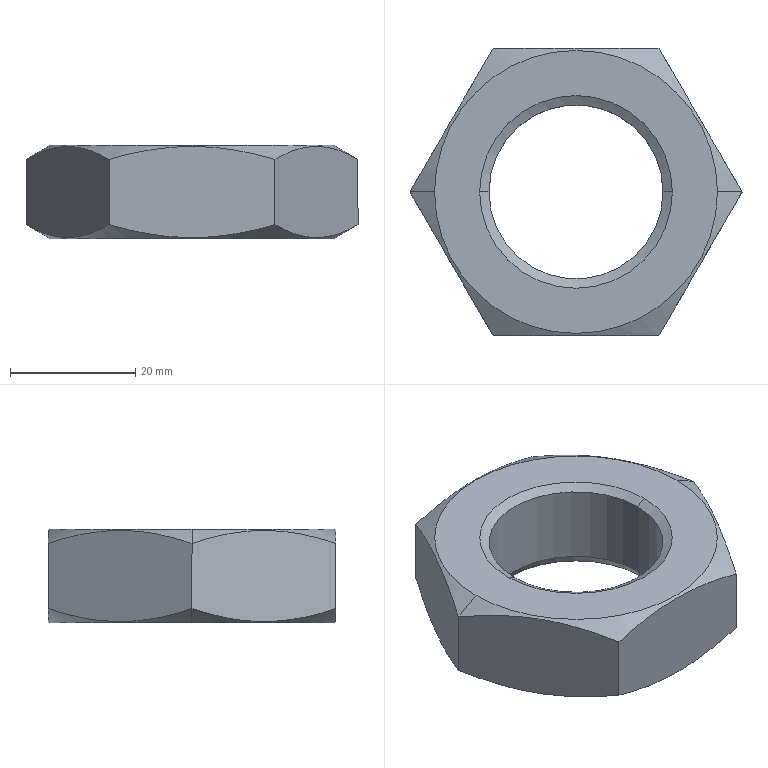Part | SolidWorks | features RevCut 2, Chamfer 1, Extrusion 1, LPattern 1 | 1 solid | 18 faces | box 53.116 x 46 x 15 mm | volume 17946 mm3 | cone 8 | plane 8 | cylinder 2 | commonest cylinder face diameters 27.835 x2
STEP:
#1=CARTESIAN_POINT('',(-13.918,0.,-0.866));
#2=VERTEX_POINT('',#1);
#3=CARTESIAN_POINT('',(13.918,0.,-0.866));
#4=VERTEX_POINT('',#3);
#5=CARTESIAN_POINT('',(0.,0.,-0.866));
#6=DIRECTION('',(0.,0.,1.));
#7=DIRECTION('',(1.,0.,0.));
#8=AXIS2_PLACEMENT_3D('',#5,#6,#7);
#9=CIRCLE('',#8,13.918);
#10=EDGE_CURVE('',#2,#4,#9,.T.);
#11=ORIENTED_EDGE('',*,*,#10,.F.);
#12=CARTESIAN_POINT('',(-15.418,0.,0.));
#13=VERTEX_POINT('',#12);
#14=CARTESIAN_POINT('',(-13.918,0.,-0.866));
#15=DIRECTION('',(-0.866,0.,0.5));
#16=VECTOR('',#15,1000.);
#17=LINE('',#14,#16);
#18=EDGE_CURVE('',#2,#13,#17,.T.);
#19=ORIENTED_EDGE('',*,*,#18,.T.);
#20=CARTESIAN_POINT('',(15.418,0.,0.));
#21=VERTEX_POINT('',#20);
#22=CARTESIAN_POINT('',(0.,0.,0.));
#23=DIRECTION('',(0.,0.,-1.));
#24=DIRECTION('',(1.,0.,0.));
#25=AXIS2_PLACEMENT_3D('',#22,#23,#24);
#26=CIRCLE('',#25,15.418);
#27=EDGE_CURVE('',#21,#13,#26,.T.);
#28=ORIENTED_EDGE('',*,*,#27,.F.);
#29=CARTESIAN_POINT('',(13.918,0.,-0.866));
#30=DIRECTION('',(0.866,0.,0.5));
#31=VECTOR('',#30,1000.);
#32=LINE('',#29,#31);
#33=EDGE_CURVE('',#4,#21,#32,.T.);
#34=ORIENTED_EDGE('',*,*,#33,.F.);
#35=EDGE_LOOP('',(#11,#19,#28,#34));
#36=FACE_OUTER_BOUND('',#35,.T.);
#37=CARTESIAN_POINT('',(0.,0.,-0.866));
#38=DIRECTION('',(0.,0.,1.));
#39=DIRECTION('',(1.,0.,0.));
#40=AXIS2_PLACEMENT_3D('',#37,#38,#39);
#41=CONICAL_SURFACE('',#40,13.918,1.047);
#42=ADVANCED_FACE('',(#36),#41,.F.);
#43=CARTESIAN_POINT('',(13.918,0.,-13.5));
#44=VERTEX_POINT('',#43);
#45=CARTESIAN_POINT('',(-13.918,0.,-13.5));
#46=VERTEX_POINT('',#45);
#47=CARTESIAN_POINT('',(0.,0.,-13.5));
#48=DIRECTION('',(0.,0.,-1.));
#49=DIRECTION('',(1.,0.,0.));
#50=AXIS2_PLACEMENT_3D('',#47,#48,#49);
#51=CIRCLE('',#50,13.918);
#52=EDGE_CURVE('',#44,#46,#51,.T.);
#53=ORIENTED_EDGE('',*,*,#52,.F.);
#54=CARTESIAN_POINT('',(14.784,0.,-15.));
#55=VERTEX_POINT('',#54);
#56=CARTESIAN_POINT('',(14.784,0.,-15.));
#57=DIRECTION('',(0.5,0.,-0.866));
#58=VECTOR('',#57,1000.);
#59=LINE('',#56,#58);
#60=EDGE_CURVE('',#44,#55,#59,.T.);
#61=ORIENTED_EDGE('',*,*,#60,.T.);
#62=CARTESIAN_POINT('',(-14.784,0.,-15.));
#63=VERTEX_POINT('',#62);
#64=CARTESIAN_POINT('',(0.,0.,-15.));
#65=DIRECTION('',(0.,0.,1.));
#66=DIRECTION('',(1.,0.,0.));
#67=AXIS2_PLACEMENT_3D('',#64,#65,#66);
#68=CIRCLE('',#67,14.784);
#69=EDGE_CURVE('',#63,#55,#68,.T.);
#70=ORIENTED_EDGE('',*,*,#69,.F.);
#71=CARTESIAN_POINT('',(-14.784,0.,-15.));
#72=DIRECTION('',(-0.5,0.,-0.866));
#73=VECTOR('',#72,1000.);
#74=LINE('',#71,#73);
#75=EDGE_CURVE('',#46,#63,#74,.T.);
#76=ORIENTED_EDGE('',*,*,#75,.F.);
#77=EDGE_LOOP('',(#53,#61,#70,#76));
#78=FACE_OUTER_BOUND('',#77,.T.);
#79=CARTESIAN_POINT('',(0.,0.,-15.));
#80=DIRECTION('',(0.,0.,-1.));
#81=DIRECTION('',(-1.,0.,0.));
#82=AXIS2_PLACEMENT_3D('',#79,#80,#81);
#83=CONICAL_SURFACE('',#82,14.784,0.5236);
#84=ADVANCED_FACE('',(#78),#83,.F.);
#85=CARTESIAN_POINT('',(-22.625,0.,0.));
#86=VERTEX_POINT('',#85);
#87=CARTESIAN_POINT('',(22.625,0.,0.));
#88=VERTEX_POINT('',#87);
#89=CARTESIAN_POINT('',(0.,0.,0.));
#90=DIRECTION('',(0.,0.,-1.));
#91=DIRECTION('',(-1.,0.,0.));
#92=AXIS2_PLACEMENT_3D('',#89,#90,#91);
#93=CIRCLE('',#92,22.625);
#94=EDGE_CURVE('',#86,#88,#93,.T.);
#95=ORIENTED_EDGE('',*,*,#94,.T.);
#96=CARTESIAN_POINT('',(26.558,0.,-2.271));
#97=VERTEX_POINT('',#96);
#98=CARTESIAN_POINT('',(22.625,0.,0.));
#99=DIRECTION('',(0.866,0.,-0.5));
#100=VECTOR('',#99,1000.);
#101=LINE('',#98,#100);
#102=EDGE_CURVE('',#88,#97,#101,.T.);
#103=ORIENTED_EDGE('',*,*,#102,.T.);
#104=CARTESIAN_POINT('',(13.279,23.,-2.271));
#105=VERTEX_POINT('',#104);
#106=CARTESIAN_POINT('',(26.558,0.,-2.271));
#107=CARTESIAN_POINT('',(25.474,1.878,-1.645));
#108=CARTESIAN_POINT('',(24.382,3.769,-1.129));
#109=CARTESIAN_POINT('',(22.175,7.591,-0.4144));
#110=CARTESIAN_POINT('',(21.06,9.523,-0.218));
#111=CARTESIAN_POINT('',(19.649,11.967,-0.2162));
#112=CARTESIAN_POINT('',(19.365,12.458,-0.2279));
#113=CARTESIAN_POINT('',(18.801,13.436,-0.2751));
#114=CARTESIAN_POINT('',(18.519,13.924,-0.3106));
#115=CARTESIAN_POINT('',(17.678,15.381,-0.4511));
#116=CARTESIAN_POINT('',(17.121,16.346,-0.5901));
#117=CARTESIAN_POINT('',(15.459,19.224,-1.127));
#118=CARTESIAN_POINT('',(14.365,21.12,-1.644));
#119=CARTESIAN_POINT('',(13.279,23.,-2.271));
#120=B_SPLINE_CURVE_WITH_KNOTS('',3,(#106,#107,#108,#109,#110,#111,#112,#113,#114,#115,#116,#117,#118,#119),.UNSPECIFIED.,.F.,.F.,(4,2,2,2,2,2,4),(0.000000238,0.006706,0.01341,0.01509,0.01676,0.02012,0.02682),.UNSPECIFIED.);
#121=EDGE_CURVE('',#97,#105,#120,.T.);
#122=ORIENTED_EDGE('',*,*,#121,.T.);
#123=CARTESIAN_POINT('',(-13.279,23.,-2.271));
#124=VERTEX_POINT('',#123);
#125=CARTESIAN_POINT('',(13.279,23.,-2.271));
#126=CARTESIAN_POINT('',(11.133,23.,-1.651));
#127=CARTESIAN_POINT('',(8.958,23.,-1.135));
#128=CARTESIAN_POINT('',(5.632,23.,-0.595));
#129=CARTESIAN_POINT('',(4.511,23.,-0.4541));
#130=CARTESIAN_POINT('',(2.252,23.,-0.2644));
#131=CARTESIAN_POINT('',(1.126,23.,-0.2166));
#132=CARTESIAN_POINT('',(-2.241,23.,-0.2163));
#133=CARTESIAN_POINT('',(-4.471,23.,-0.409));
#134=CARTESIAN_POINT('',(-7.797,23.,-0.9453));
#135=CARTESIAN_POINT('',(-8.904,23.,-1.165));
#136=CARTESIAN_POINT('',(-11.109,23.,-1.673));
#137=CARTESIAN_POINT('',(-12.199,23.,-1.959));
#138=CARTESIAN_POINT('',(-13.279,23.,-2.271));
#139=B_SPLINE_CURVE_WITH_KNOTS('',3,(#125,#126,#127,#128,#129,#130,#131,#132,#133,#134,#135,#136,#137,#138),.UNSPECIFIED.,.F.,.F.,(4,2,2,2,2,2,4),(0.00977,0.01647,0.01982,0.02317,0.02987,0.03323,0.03658),.UNSPECIFIED.);
#140=EDGE_CURVE('',#105,#124,#139,.T.);
#141=ORIENTED_EDGE('',*,*,#140,.T.);
#142=CARTESIAN_POINT('',(-26.558,0.,-2.271));
#143=VERTEX_POINT('',#142);
#144=CARTESIAN_POINT('',(-13.279,23.,-2.271));
#145=CARTESIAN_POINT('',(-14.363,21.122,-1.645));
#146=CARTESIAN_POINT('',(-15.455,19.231,-1.129));
#147=CARTESIAN_POINT('',(-17.662,15.409,-0.4144));
#148=CARTESIAN_POINT('',(-18.777,13.477,-0.218));
#149=CARTESIAN_POINT('',(-20.188,11.033,-0.2162));
#150=CARTESIAN_POINT('',(-20.472,10.542,-0.2279));
#151=CARTESIAN_POINT('',(-21.037,9.564,-0.2751));
#152=CARTESIAN_POINT('',(-21.318,9.076,-0.3106));
#153=CARTESIAN_POINT('',(-22.159,7.619,-0.4511));
#154=CARTESIAN_POINT('',(-22.717,6.654,-0.5901));
#155=CARTESIAN_POINT('',(-24.378,3.776,-1.127));
#156=CARTESIAN_POINT('',(-25.473,1.88,-1.644));
#157=CARTESIAN_POINT('',(-26.558,0.,-2.271));
#158=B_SPLINE_CURVE_WITH_KNOTS('',3,(#144,#145,#146,#147,#148,#149,#150,#151,#152,#153,#154,#155,#156,#157),.UNSPECIFIED.,.F.,.F.,(4,2,2,2,2,2,4),(0.000000238,0.006706,0.01341,0.01509,0.01676,0.02012,0.02682),.UNSPECIFIED.);
#159=EDGE_CURVE('',#124,#143,#158,.T.);
#160=ORIENTED_EDGE('',*,*,#159,.T.);
#161=CARTESIAN_POINT('',(-22.625,0.,0.));
#162=DIRECTION('',(-0.866,0.,-0.5));
#163=VECTOR('',#162,1000.);
#164=LINE('',#161,#163);
#165=EDGE_CURVE('',#86,#143,#164,.T.);
#166=ORIENTED_EDGE('',*,*,#165,.F.);
#167=EDGE_LOOP('',(#95,#103,#122,#141,#160,#166));
#168=FACE_OUTER_BOUND('',#167,.T.);
#169=CARTESIAN_POINT('',(0.,0.,0.));
#170=DIRECTION('',(0.,0.,-1.));
#171=DIRECTION('',(-1.,0.,0.));
#172=AXIS2_PLACEMENT_3D('',#169,#170,#171);
#173=CONICAL_SURFACE('',#172,22.625,1.047);
#174=ADVANCED_FACE('',(#168),#173,.T.);
#175=CARTESIAN_POINT('',(-22.625,0.,-15.));
#176=VERTEX_POINT('',#175);
#177=CARTESIAN_POINT('',(22.625,0.,-15.));
#178=VERTEX_POINT('',#177);
#179=CARTESIAN_POINT('',(0.,0.,-15.));
#180=DIRECTION('',(0.,0.,-1.));
#181=DIRECTION('',(-1.,0.,0.));
#182=AXIS2_PLACEMENT_3D('',#179,#180,#181);
#183=CIRCLE('',#182,22.625);
#184=EDGE_CURVE('',#176,#178,#183,.T.);
#185=ORIENTED_EDGE('',*,*,#184,.F.);
#186=CARTESIAN_POINT('',(-26.558,0.,-12.729));
#187=VERTEX_POINT('',#186);
#188=CARTESIAN_POINT('',(-26.558,0.,-12.729));
#189=DIRECTION('',(-0.866,0.,0.5));
#190=VECTOR('',#189,1000.);
#191=LINE('',#188,#190);
#192=EDGE_CURVE('',#176,#187,#191,.T.);
#193=ORIENTED_EDGE('',*,*,#192,.T.);
#194=CARTESIAN_POINT('',(-13.279,23.,-12.729));
#195=VERTEX_POINT('',#194);
#196=CARTESIAN_POINT('',(-26.558,0.,-12.729));
#197=CARTESIAN_POINT('',(-25.474,1.878,-13.355));
#198=CARTESIAN_POINT('',(-24.382,3.769,-13.871));
#199=CARTESIAN_POINT('',(-22.175,7.591,-14.586));
#200=CARTESIAN_POINT('',(-21.06,9.523,-14.782));
#201=CARTESIAN_POINT('',(-19.649,11.967,-14.784));
#202=CARTESIAN_POINT('',(-19.365,12.458,-14.772));
#203=CARTESIAN_POINT('',(-18.801,13.436,-14.725));
#204=CARTESIAN_POINT('',(-18.519,13.924,-14.689));
#205=CARTESIAN_POINT('',(-17.678,15.381,-14.549));
#206=CARTESIAN_POINT('',(-17.121,16.346,-14.41));
#207=CARTESIAN_POINT('',(-15.459,19.224,-13.873));
#208=CARTESIAN_POINT('',(-14.365,21.12,-13.356));
#209=CARTESIAN_POINT('',(-13.279,23.,-12.729));
#210=B_SPLINE_CURVE_WITH_KNOTS('',3,(#196,#197,#198,#199,#200,#201,#202,#203,#204,#205,#206,#207,#208,#209),.UNSPECIFIED.,.F.,.F.,(4,2,2,2,2,2,4),(0.000000238,0.006706,0.01341,0.01509,0.01676,0.02012,0.02682),.UNSPECIFIED.);
#211=EDGE_CURVE('',#187,#195,#210,.T.);
#212=ORIENTED_EDGE('',*,*,#211,.T.);
#213=CARTESIAN_POINT('',(13.279,23.,-12.729));
#214=VERTEX_POINT('',#213);
#215=CARTESIAN_POINT('',(-13.279,23.,-12.729));
#216=CARTESIAN_POINT('',(-12.199,23.,-13.041));
#217=CARTESIAN_POINT('',(-11.109,23.,-13.327));
#218=CARTESIAN_POINT('',(-8.904,23.,-13.835));
#219=CARTESIAN_POINT('',(-7.797,23.,-14.055));
#220=CARTESIAN_POINT('',(-4.471,23.,-14.591));
#221=CARTESIAN_POINT('',(-2.241,23.,-14.784));
#222=CARTESIAN_POINT('',(1.126,23.,-14.783));
#223=CARTESIAN_POINT('',(2.252,23.,-14.736));
#224=CARTESIAN_POINT('',(4.511,23.,-14.546));
#225=CARTESIAN_POINT('',(5.632,23.,-14.405));
#226=CARTESIAN_POINT('',(8.958,23.,-13.865));
#227=CARTESIAN_POINT('',(11.133,23.,-13.349));
#228=CARTESIAN_POINT('',(13.279,23.,-12.729));
#229=B_SPLINE_CURVE_WITH_KNOTS('',3,(#215,#216,#217,#218,#219,#220,#221,#222,#223,#224,#225,#226,#227,#228),.UNSPECIFIED.,.F.,.F.,(4,2,2,2,2,2,4),(0.02366,0.02702,0.03038,0.0371,0.04045,0.04381,0.05053),.UNSPECIFIED.);
#230=EDGE_CURVE('',#195,#214,#229,.T.);
#231=ORIENTED_EDGE('',*,*,#230,.T.);
#232=CARTESIAN_POINT('',(26.558,0.,-12.729));
#233=VERTEX_POINT('',#232);
#234=CARTESIAN_POINT('',(13.279,23.,-12.729));
#235=CARTESIAN_POINT('',(14.363,21.122,-13.355));
#236=CARTESIAN_POINT('',(15.455,19.231,-13.871));
#237=CARTESIAN_POINT('',(17.662,15.409,-14.586));
#238=CARTESIAN_POINT('',(18.777,13.477,-14.782));
#239=CARTESIAN_POINT('',(20.188,11.033,-14.784));
#240=CARTESIAN_POINT('',(20.472,10.542,-14.772));
#241=CARTESIAN_POINT('',(21.037,9.564,-14.725));
#242=CARTESIAN_POINT('',(21.318,9.076,-14.689));
#243=CARTESIAN_POINT('',(22.159,7.619,-14.549));
#244=CARTESIAN_POINT('',(22.717,6.654,-14.41));
#245=CARTESIAN_POINT('',(24.378,3.776,-13.873));
#246=CARTESIAN_POINT('',(25.473,1.88,-13.356));
#247=CARTESIAN_POINT('',(26.558,0.,-12.729));
#248=B_SPLINE_CURVE_WITH_KNOTS('',3,(#234,#235,#236,#237,#238,#239,#240,#241,#242,#243,#244,#245,#246,#247),.UNSPECIFIED.,.F.,.F.,(4,2,2,2,2,2,4),(0.000000238,0.006706,0.01341,0.01509,0.01676,0.02012,0.02682),.UNSPECIFIED.);
#249=EDGE_CURVE('',#214,#233,#248,.T.);
#250=ORIENTED_EDGE('',*,*,#249,.T.);
#251=CARTESIAN_POINT('',(26.558,0.,-12.729));
#252=DIRECTION('',(0.866,0.,0.5));
#253=VECTOR('',#252,1000.);
#254=LINE('',#251,#253);
#255=EDGE_CURVE('',#178,#233,#254,.T.);
#256=ORIENTED_EDGE('',*,*,#255,.F.);
#257=EDGE_LOOP('',(#185,#193,#212,#231,#250,#256));
#258=FACE_OUTER_BOUND('',#257,.T.);
#259=CARTESIAN_POINT('',(0.,0.,-12.729));
#260=DIRECTION('',(0.,0.,1.));
#261=DIRECTION('',(1.,0.,0.));
#262=AXIS2_PLACEMENT_3D('',#259,#260,#261);
#263=CONICAL_SURFACE('',#262,26.558,1.047);
#264=ADVANCED_FACE('',(#258),#263,.T.);
#265=ORIENTED_EDGE('',*,*,#52,.T.);
#266=CARTESIAN_POINT('',(-13.918,0.,-15.));
#267=DIRECTION('',(0.,0.,1.));
#268=VECTOR('',#267,1000.);
#269=LINE('',#266,#268);
#270=EDGE_CURVE('',#46,#2,#269,.T.);
#271=ORIENTED_EDGE('',*,*,#270,.T.);
#272=ORIENTED_EDGE('',*,*,#10,.T.);
#273=CARTESIAN_POINT('',(13.918,0.,-15.));
#274=DIRECTION('',(0.,0.,1.));
#275=VECTOR('',#274,1000.);
#276=LINE('',#273,#275);
#277=EDGE_CURVE('',#44,#4,#276,.T.);
#278=ORIENTED_EDGE('',*,*,#277,.F.);
#279=EDGE_LOOP('',(#265,#271,#272,#278));
#280=FACE_OUTER_BOUND('',#279,.T.);
#281=CARTESIAN_POINT('',(0.,0.,-15.));
#282=DIRECTION('',(0.,0.,1.));
#283=DIRECTION('',(1.,0.,0.));
#284=AXIS2_PLACEMENT_3D('',#281,#282,#283);
#285=CYLINDRICAL_SURFACE('',#284,13.918);
#286=ADVANCED_FACE('',(#280),#285,.F.);
#287=CARTESIAN_POINT('',(-13.279,-23.,-2.271));
#288=VERTEX_POINT('',#287);
#289=CARTESIAN_POINT('',(13.279,-23.,-2.271));
#290=VERTEX_POINT('',#289);
#291=CARTESIAN_POINT('',(-13.279,-23.,-2.271));
#292=CARTESIAN_POINT('',(-12.199,-23.,-1.959));
#293=CARTESIAN_POINT('',(-11.109,-23.,-1.673));
#294=CARTESIAN_POINT('',(-8.904,-23.,-1.165));
#295=CARTESIAN_POINT('',(-7.797,-23.,-0.9453));
#296=CARTESIAN_POINT('',(-4.471,-23.,-0.409));
#297=CARTESIAN_POINT('',(-2.241,-23.,-0.2163));
#298=CARTESIAN_POINT('',(1.126,-23.,-0.2166));
#299=CARTESIAN_POINT('',(2.252,-23.,-0.2644));
#300=CARTESIAN_POINT('',(4.511,-23.,-0.4541));
#301=CARTESIAN_POINT('',(5.632,-23.,-0.595));
#302=CARTESIAN_POINT('',(8.958,-23.,-1.135));
#303=CARTESIAN_POINT('',(11.133,-23.,-1.651));
#304=CARTESIAN_POINT('',(13.279,-23.,-2.271));
#305=B_SPLINE_CURVE_WITH_KNOTS('',3,(#291,#292,#293,#294,#295,#296,#297,#298,#299,#300,#301,#302,#303,#304),.UNSPECIFIED.,.F.,.F.,(4,2,2,2,2,2,4),(0.02366,0.02702,0.03038,0.0371,0.04045,0.04381,0.05053),.UNSPECIFIED.);
#306=EDGE_CURVE('',#288,#290,#305,.T.);
#307=ORIENTED_EDGE('',*,*,#306,.F.);
#308=CARTESIAN_POINT('',(-13.279,-23.,-12.729));
#309=VERTEX_POINT('',#308);
#310=CARTESIAN_POINT('',(-13.279,-23.,-15.));
#311=DIRECTION('',(0.,0.,1.));
#312=VECTOR('',#311,1000.);
#313=LINE('',#310,#312);
#314=EDGE_CURVE('',#309,#288,#313,.T.);
#315=ORIENTED_EDGE('',*,*,#314,.F.);
#316=CARTESIAN_POINT('',(13.279,-23.,-12.729));
#317=VERTEX_POINT('',#316);
#318=CARTESIAN_POINT('',(13.279,-23.,-12.729));
#319=CARTESIAN_POINT('',(11.133,-23.,-13.349));
#320=CARTESIAN_POINT('',(8.958,-23.,-13.865));
#321=CARTESIAN_POINT('',(5.632,-23.,-14.405));
#322=CARTESIAN_POINT('',(4.511,-23.,-14.546));
#323=CARTESIAN_POINT('',(2.252,-23.,-14.736));
#324=CARTESIAN_POINT('',(1.126,-23.,-14.783));
#325=CARTESIAN_POINT('',(-2.241,-23.,-14.784));
#326=CARTESIAN_POINT('',(-4.471,-23.,-14.591));
#327=CARTESIAN_POINT('',(-7.797,-23.,-14.055));
#328=CARTESIAN_POINT('',(-8.904,-23.,-13.835));
#329=CARTESIAN_POINT('',(-11.109,-23.,-13.327));
#330=CARTESIAN_POINT('',(-12.199,-23.,-13.041));
#331=CARTESIAN_POINT('',(-13.279,-23.,-12.729));
#332=B_SPLINE_CURVE_WITH_KNOTS('',3,(#318,#319,#320,#321,#322,#323,#324,#325,#326,#327,#328,#329,#330,#331),.UNSPECIFIED.,.F.,.F.,(4,2,2,2,2,2,4),(0.00977,0.01647,0.01982,0.02317,0.02987,0.03323,0.03658),.UNSPECIFIED.);
#333=EDGE_CURVE('',#317,#309,#332,.T.);
#334=ORIENTED_EDGE('',*,*,#333,.F.);
#335=CARTESIAN_POINT('',(13.279,-23.,-15.));
#336=DIRECTION('',(0.,0.,1.));
#337=VECTOR('',#336,1000.);
#338=LINE('',#335,#337);
#339=EDGE_CURVE('',#317,#290,#338,.T.);
#340=ORIENTED_EDGE('',*,*,#339,.T.);
#341=EDGE_LOOP('',(#307,#315,#334,#340));
#342=FACE_OUTER_BOUND('',#341,.T.);
#343=CARTESIAN_POINT('',(-13.279,-23.,-15.));
#344=DIRECTION('',(0.,-1.,0.));
#345=DIRECTION('',(0.,0.,-1.));
#346=AXIS2_PLACEMENT_3D('',#343,#344,#345);
#347=PLANE('',#346);
#348=ADVANCED_FACE('',(#342),#347,.T.);
#349=CARTESIAN_POINT('',(-26.558,0.,-2.271));
#350=CARTESIAN_POINT('',(-25.474,-1.878,-1.645));
#351=CARTESIAN_POINT('',(-24.382,-3.769,-1.129));
#352=CARTESIAN_POINT('',(-22.175,-7.591,-0.4144));
#353=CARTESIAN_POINT('',(-21.06,-9.523,-0.218));
#354=CARTESIAN_POINT('',(-19.649,-11.967,-0.2162));
#355=CARTESIAN_POINT('',(-19.365,-12.458,-0.2279));
#356=CARTESIAN_POINT('',(-18.801,-13.436,-0.2751));
#357=CARTESIAN_POINT('',(-18.519,-13.924,-0.3106));
#358=CARTESIAN_POINT('',(-17.678,-15.381,-0.4511));
#359=CARTESIAN_POINT('',(-17.121,-16.346,-0.5901));
#360=CARTESIAN_POINT('',(-15.459,-19.224,-1.127));
#361=CARTESIAN_POINT('',(-14.365,-21.12,-1.644));
#362=CARTESIAN_POINT('',(-13.279,-23.,-2.271));
#363=B_SPLINE_CURVE_WITH_KNOTS('',3,(#349,#350,#351,#352,#353,#354,#355,#356,#357,#358,#359,#360,#361,#362),.UNSPECIFIED.,.F.,.F.,(4,2,2,2,2,2,4),(0.000000238,0.006706,0.01341,0.01509,0.01676,0.02012,0.02682),.UNSPECIFIED.);
#364=EDGE_CURVE('',#143,#288,#363,.T.);
#365=ORIENTED_EDGE('',*,*,#364,.F.);
#366=CARTESIAN_POINT('',(-26.558,0.,-15.));
#367=DIRECTION('',(0.,0.,1.));
#368=VECTOR('',#367,1000.);
#369=LINE('',#366,#368);
#370=EDGE_CURVE('',#187,#143,#369,.T.);
#371=ORIENTED_EDGE('',*,*,#370,.F.);
#372=CARTESIAN_POINT('',(-13.279,-23.,-12.729));
#373=CARTESIAN_POINT('',(-14.363,-21.122,-13.355));
#374=CARTESIAN_POINT('',(-15.455,-19.231,-13.871));
#375=CARTESIAN_POINT('',(-17.662,-15.409,-14.586));
#376=CARTESIAN_POINT('',(-18.777,-13.477,-14.782));
#377=CARTESIAN_POINT('',(-20.188,-11.033,-14.784));
#378=CARTESIAN_POINT('',(-20.472,-10.542,-14.772));
#379=CARTESIAN_POINT('',(-21.037,-9.564,-14.725));
#380=CARTESIAN_POINT('',(-21.318,-9.076,-14.689));
#381=CARTESIAN_POINT('',(-22.159,-7.619,-14.549));
#382=CARTESIAN_POINT('',(-22.717,-6.654,-14.41));
#383=CARTESIAN_POINT('',(-24.378,-3.776,-13.873));
#384=CARTESIAN_POINT('',(-25.473,-1.88,-13.356));
#385=CARTESIAN_POINT('',(-26.558,0.,-12.729));
#386=B_SPLINE_CURVE_WITH_KNOTS('',3,(#372,#373,#374,#375,#376,#377,#378,#379,#380,#381,#382,#383,#384,#385),.UNSPECIFIED.,.F.,.F.,(4,2,2,2,2,2,4),(0.000000238,0.006706,0.01341,0.01509,0.01676,0.02012,0.02682),.UNSPECIFIED.);
#387=EDGE_CURVE('',#309,#187,#386,.T.);
#388=ORIENTED_EDGE('',*,*,#387,.F.);
#389=ORIENTED_EDGE('',*,*,#314,.T.);
#390=EDGE_LOOP('',(#365,#371,#388,#389));
#391=FACE_OUTER_BOUND('',#390,.T.);
#392=CARTESIAN_POINT('',(-26.558,0.,-15.));
#393=DIRECTION('',(-0.866,-0.5,0.));
#394=DIRECTION('',(0.5,-0.866,0.));
#395=AXIS2_PLACEMENT_3D('',#392,#393,#394);
#396=PLANE('',#395);
#397=ADVANCED_FACE('',(#391),#396,.T.);
#398=ORIENTED_EDGE('',*,*,#159,.F.);
#399=CARTESIAN_POINT('',(-13.279,23.,-15.));
#400=DIRECTION('',(0.,0.,1.));
#401=VECTOR('',#400,1000.);
#402=LINE('',#399,#401);
#403=EDGE_CURVE('',#195,#124,#402,.T.);
#404=ORIENTED_EDGE('',*,*,#403,.F.);
#405=ORIENTED_EDGE('',*,*,#211,.F.);
#406=ORIENTED_EDGE('',*,*,#370,.T.);
#407=EDGE_LOOP('',(#398,#404,#405,#406));
#408=FACE_OUTER_BOUND('',#407,.T.);
#409=CARTESIAN_POINT('',(-13.279,23.,-15.));
#410=DIRECTION('',(-0.866,0.5,0.));
#411=DIRECTION('',(-0.5,-0.866,0.));
#412=AXIS2_PLACEMENT_3D('',#409,#410,#411);
#413=PLANE('',#412);
#414=ADVANCED_FACE('',(#408),#413,.T.);
#415=ORIENTED_EDGE('',*,*,#140,.F.);
#416=CARTESIAN_POINT('',(13.279,23.,-15.));
#417=DIRECTION('',(0.,0.,1.));
#418=VECTOR('',#417,1000.);
#419=LINE('',#416,#418);
#420=EDGE_CURVE('',#214,#105,#419,.T.);
#421=ORIENTED_EDGE('',*,*,#420,.F.);
#422=ORIENTED_EDGE('',*,*,#230,.F.);
#423=ORIENTED_EDGE('',*,*,#403,.T.);
#424=EDGE_LOOP('',(#415,#421,#422,#423));
#425=FACE_OUTER_BOUND('',#424,.T.);
#426=CARTESIAN_POINT('',(13.279,23.,-15.));
#427=DIRECTION('',(0.,1.,0.));
#428=DIRECTION('',(0.,0.,1.));
#429=AXIS2_PLACEMENT_3D('',#426,#427,#428);
#430=PLANE('',#429);
#431=ADVANCED_FACE('',(#425),#430,.T.);
#432=ORIENTED_EDGE('',*,*,#121,.F.);
#433=CARTESIAN_POINT('',(26.558,0.,-15.));
#434=DIRECTION('',(0.,0.,1.));
#435=VECTOR('',#434,1000.);
#436=LINE('',#433,#435);
#437=EDGE_CURVE('',#233,#97,#436,.T.);
#438=ORIENTED_EDGE('',*,*,#437,.F.);
#439=ORIENTED_EDGE('',*,*,#249,.F.);
#440=ORIENTED_EDGE('',*,*,#420,.T.);
#441=EDGE_LOOP('',(#432,#438,#439,#440));
#442=FACE_OUTER_BOUND('',#441,.T.);
#443=CARTESIAN_POINT('',(26.558,0.,-15.));
#444=DIRECTION('',(0.866,0.5,0.));
#445=DIRECTION('',(-0.5,0.866,0.));
#446=AXIS2_PLACEMENT_3D('',#443,#444,#445);
#447=PLANE('',#446);
#448=ADVANCED_FACE('',(#442),#447,.T.);
#449=CARTESIAN_POINT('',(13.279,-23.,-2.271));
#450=CARTESIAN_POINT('',(14.363,-21.122,-1.645));
#451=CARTESIAN_POINT('',(15.455,-19.231,-1.129));
#452=CARTESIAN_POINT('',(17.662,-15.409,-0.4144));
#453=CARTESIAN_POINT('',(18.777,-13.477,-0.218));
#454=CARTESIAN_POINT('',(20.188,-11.033,-0.2162));
#455=CARTESIAN_POINT('',(20.472,-10.542,-0.2279));
#456=CARTESIAN_POINT('',(21.037,-9.564,-0.2751));
#457=CARTESIAN_POINT('',(21.318,-9.076,-0.3106));
#458=CARTESIAN_POINT('',(22.159,-7.619,-0.4511));
#459=CARTESIAN_POINT('',(22.717,-6.654,-0.5901));
#460=CARTESIAN_POINT('',(24.378,-3.776,-1.127));
#461=CARTESIAN_POINT('',(25.473,-1.88,-1.644));
#462=CARTESIAN_POINT('',(26.558,0.,-2.271));
#463=B_SPLINE_CURVE_WITH_KNOTS('',3,(#449,#450,#451,#452,#453,#454,#455,#456,#457,#458,#459,#460,#461,#462),.UNSPECIFIED.,.F.,.F.,(4,2,2,2,2,2,4),(0.000000238,0.006706,0.01341,0.01509,0.01676,0.02012,0.02682),.UNSPECIFIED.);
#464=EDGE_CURVE('',#290,#97,#463,.T.);
#465=ORIENTED_EDGE('',*,*,#464,.F.);
#466=ORIENTED_EDGE('',*,*,#339,.F.);
#467=CARTESIAN_POINT('',(26.558,0.,-12.729));
#468=CARTESIAN_POINT('',(25.474,-1.878,-13.355));
#469=CARTESIAN_POINT('',(24.382,-3.769,-13.871));
#470=CARTESIAN_POINT('',(22.175,-7.591,-14.586));
#471=CARTESIAN_POINT('',(21.06,-9.523,-14.782));
#472=CARTESIAN_POINT('',(19.649,-11.967,-14.784));
#473=CARTESIAN_POINT('',(19.365,-12.458,-14.772));
#474=CARTESIAN_POINT('',(18.801,-13.436,-14.725));
#475=CARTESIAN_POINT('',(18.519,-13.924,-14.689));
#476=CARTESIAN_POINT('',(17.678,-15.381,-14.549));
#477=CARTESIAN_POINT('',(17.121,-16.346,-14.41));
#478=CARTESIAN_POINT('',(15.459,-19.224,-13.873));
#479=CARTESIAN_POINT('',(14.365,-21.12,-13.356));
#480=CARTESIAN_POINT('',(13.279,-23.,-12.729));
#481=B_SPLINE_CURVE_WITH_KNOTS('',3,(#467,#468,#469,#470,#471,#472,#473,#474,#475,#476,#477,#478,#479,#480),.UNSPECIFIED.,.F.,.F.,(4,2,2,2,2,2,4),(0.000000238,0.006706,0.01341,0.01509,0.01676,0.02012,0.02682),.UNSPECIFIED.);
#482=EDGE_CURVE('',#233,#317,#481,.T.);
#483=ORIENTED_EDGE('',*,*,#482,.F.);
#484=ORIENTED_EDGE('',*,*,#437,.T.);
#485=EDGE_LOOP('',(#465,#466,#483,#484));
#486=FACE_OUTER_BOUND('',#485,.T.);
#487=CARTESIAN_POINT('',(13.279,-23.,-15.));
#488=DIRECTION('',(0.866,-0.5,0.));
#489=DIRECTION('',(0.5,0.866,0.));
#490=AXIS2_PLACEMENT_3D('',#487,#488,#489);
#491=PLANE('',#490);
#492=ADVANCED_FACE('',(#486),#491,.T.);
#493=ORIENTED_EDGE('',*,*,#69,.T.);
#494=CARTESIAN_POINT('',(0.,0.,-15.));
#495=DIRECTION('',(0.,0.,1.));
#496=DIRECTION('',(1.,0.,0.));
#497=AXIS2_PLACEMENT_3D('',#494,#495,#496);
#498=CIRCLE('',#497,14.784);
#499=EDGE_CURVE('',#55,#63,#498,.T.);
#500=ORIENTED_EDGE('',*,*,#499,.T.);
#501=EDGE_LOOP('',(#493,#500));
#502=FACE_BOUND('',#501,.T.);
#503=CARTESIAN_POINT('',(0.,0.,-15.));
#504=DIRECTION('',(0.,0.,-1.));
#505=DIRECTION('',(-1.,0.,0.));
#506=AXIS2_PLACEMENT_3D('',#503,#504,#505);
#507=CIRCLE('',#506,22.625);
#508=EDGE_CURVE('',#178,#176,#507,.T.);
#509=ORIENTED_EDGE('',*,*,#508,.T.);
#510=ORIENTED_EDGE('',*,*,#184,.T.);
#511=EDGE_LOOP('',(#509,#510));
#512=FACE_OUTER_BOUND('',#511,.T.);
#513=CARTESIAN_POINT('',(13.279,-23.,-15.));
#514=DIRECTION('',(0.,0.,1.));
#515=DIRECTION('',(1.,0.,0.));
#516=AXIS2_PLACEMENT_3D('',#513,#514,#515);
#517=PLANE('',#516);
#518=ADVANCED_FACE('',(#502,#512),#517,.F.);
#519=ORIENTED_EDGE('',*,*,#27,.T.);
#520=CARTESIAN_POINT('',(0.,0.,0.));
#521=DIRECTION('',(0.,0.,-1.));
#522=DIRECTION('',(1.,0.,0.));
#523=AXIS2_PLACEMENT_3D('',#520,#521,#522);
#524=CIRCLE('',#523,15.418);
#525=EDGE_CURVE('',#13,#21,#524,.T.);
#526=ORIENTED_EDGE('',*,*,#525,.T.);
#527=EDGE_LOOP('',(#519,#526));
#528=FACE_BOUND('',#527,.T.);
#529=ORIENTED_EDGE('',*,*,#94,.F.);
#530=CARTESIAN_POINT('',(0.,0.,0.));
#531=DIRECTION('',(0.,0.,-1.));
#532=DIRECTION('',(-1.,0.,0.));
#533=AXIS2_PLACEMENT_3D('',#530,#531,#532);
#534=CIRCLE('',#533,22.625);
#535=EDGE_CURVE('',#88,#86,#534,.T.);
#536=ORIENTED_EDGE('',*,*,#535,.F.);
#537=EDGE_LOOP('',(#529,#536));
#538=FACE_OUTER_BOUND('',#537,.T.);
#539=CARTESIAN_POINT('',(13.279,-23.,0.));
#540=DIRECTION('',(0.,0.,1.));
#541=DIRECTION('',(1.,0.,0.));
#542=AXIS2_PLACEMENT_3D('',#539,#540,#541);
#543=PLANE('',#542);
#544=ADVANCED_FACE('',(#528,#538),#543,.T.);
#545=ORIENTED_EDGE('',*,*,#270,.F.);
#546=CARTESIAN_POINT('',(0.,0.,-13.5));
#547=DIRECTION('',(0.,0.,-1.));
#548=DIRECTION('',(1.,0.,0.));
#549=AXIS2_PLACEMENT_3D('',#546,#547,#548);
#550=CIRCLE('',#549,13.918);
#551=EDGE_CURVE('',#46,#44,#550,.T.);
#552=ORIENTED_EDGE('',*,*,#551,.T.);
#553=ORIENTED_EDGE('',*,*,#277,.T.);
#554=CARTESIAN_POINT('',(0.,0.,-0.866));
#555=DIRECTION('',(0.,0.,1.));
#556=DIRECTION('',(1.,0.,0.));
#557=AXIS2_PLACEMENT_3D('',#554,#555,#556);
#558=CIRCLE('',#557,13.918);
#559=EDGE_CURVE('',#4,#2,#558,.T.);
#560=ORIENTED_EDGE('',*,*,#559,.T.);
#561=EDGE_LOOP('',(#545,#552,#553,#560));
#562=FACE_OUTER_BOUND('',#561,.T.);
#563=CARTESIAN_POINT('',(0.,0.,-15.));
#564=DIRECTION('',(0.,0.,1.));
#565=DIRECTION('',(1.,0.,0.));
#566=AXIS2_PLACEMENT_3D('',#563,#564,#565);
#567=CYLINDRICAL_SURFACE('',#566,13.918);
#568=ADVANCED_FACE('',(#562),#567,.F.);
#569=ORIENTED_EDGE('',*,*,#192,.F.);
#570=ORIENTED_EDGE('',*,*,#508,.F.);
#571=ORIENTED_EDGE('',*,*,#255,.T.);
#572=ORIENTED_EDGE('',*,*,#482,.T.);
#573=ORIENTED_EDGE('',*,*,#333,.T.);
#574=ORIENTED_EDGE('',*,*,#387,.T.);
#575=EDGE_LOOP('',(#569,#570,#571,#572,#573,#574));
#576=FACE_OUTER_BOUND('',#575,.T.);
#577=CARTESIAN_POINT('',(0.,0.,-12.729));
#578=DIRECTION('',(0.,0.,1.));
#579=DIRECTION('',(1.,0.,0.));
#580=AXIS2_PLACEMENT_3D('',#577,#578,#579);
#581=CONICAL_SURFACE('',#580,26.558,1.047);
#582=ADVANCED_FACE('',(#576),#581,.T.);
#583=ORIENTED_EDGE('',*,*,#102,.F.);
#584=ORIENTED_EDGE('',*,*,#535,.T.);
#585=ORIENTED_EDGE('',*,*,#165,.T.);
#586=ORIENTED_EDGE('',*,*,#364,.T.);
#587=ORIENTED_EDGE('',*,*,#306,.T.);
#588=ORIENTED_EDGE('',*,*,#464,.T.);
#589=EDGE_LOOP('',(#583,#584,#585,#586,#587,#588));
#590=FACE_OUTER_BOUND('',#589,.T.);
#591=CARTESIAN_POINT('',(0.,0.,0.));
#592=DIRECTION('',(0.,0.,-1.));
#593=DIRECTION('',(-1.,0.,0.));
#594=AXIS2_PLACEMENT_3D('',#591,#592,#593);
#595=CONICAL_SURFACE('',#594,22.625,1.047);
#596=ADVANCED_FACE('',(#590),#595,.T.);
#597=ORIENTED_EDGE('',*,*,#60,.F.);
#598=ORIENTED_EDGE('',*,*,#551,.F.);
#599=ORIENTED_EDGE('',*,*,#75,.T.);
#600=ORIENTED_EDGE('',*,*,#499,.F.);
#601=EDGE_LOOP('',(#597,#598,#599,#600));
#602=FACE_OUTER_BOUND('',#601,.T.);
#603=CARTESIAN_POINT('',(0.,0.,-15.));
#604=DIRECTION('',(0.,0.,-1.));
#605=DIRECTION('',(-1.,0.,0.));
#606=AXIS2_PLACEMENT_3D('',#603,#604,#605);
#607=CONICAL_SURFACE('',#606,14.784,0.5236);
#608=ADVANCED_FACE('',(#602),#607,.F.);
#609=ORIENTED_EDGE('',*,*,#18,.F.);
#610=ORIENTED_EDGE('',*,*,#559,.F.);
#611=ORIENTED_EDGE('',*,*,#33,.T.);
#612=ORIENTED_EDGE('',*,*,#525,.F.);
#613=EDGE_LOOP('',(#609,#610,#611,#612));
#614=FACE_OUTER_BOUND('',#613,.T.);
#615=CARTESIAN_POINT('',(0.,0.,-0.866));
#616=DIRECTION('',(0.,0.,1.));
#617=DIRECTION('',(1.,0.,0.));
#618=AXIS2_PLACEMENT_3D('',#615,#616,#617);
#619=CONICAL_SURFACE('',#618,13.918,1.047);
#620=ADVANCED_FACE('',(#614),#619,.F.);
#621=CLOSED_SHELL('',(#42,#84,#174,#264,#286,#348,#397,#414,#431,#448,#492,#518,#544,#568,#582,#596,#608,#620));
#622=MANIFOLD_SOLID_BREP('',#621);
#623=CARTESIAN_POINT('',(0.,0.,0.));
#624=DIRECTION('',(0.,0.,1.));
#625=DIRECTION('',(1.,0.,0.));
#626=AXIS2_PLACEMENT_3D('',#623,#624,#625);
#627=(LENGTH_UNIT()NAMED_UNIT(*)SI_UNIT(.MILLI.,.METRE.));
#628=UNCERTAINTY_MEASURE_WITH_UNIT(LENGTH_MEASURE(0.00001),#627,'','');
#629=(NAMED_UNIT(*)PLANE_ANGLE_UNIT()SI_UNIT($,.RADIAN.));
#630=(NAMED_UNIT(*)SI_UNIT($,.STERADIAN.)SOLID_ANGLE_UNIT());
#631=(GEOMETRIC_REPRESENTATION_CONTEXT(3)GLOBAL_UNCERTAINTY_ASSIGNED_CONTEXT((#628))GLOBAL_UNIT_ASSIGNED_CONTEXT((#627,#629,#630))REPRESENTATION_CONTEXT('',''));
#632=ADVANCED_BREP_SHAPE_REPRESENTATION('',(#622,#626),#631);